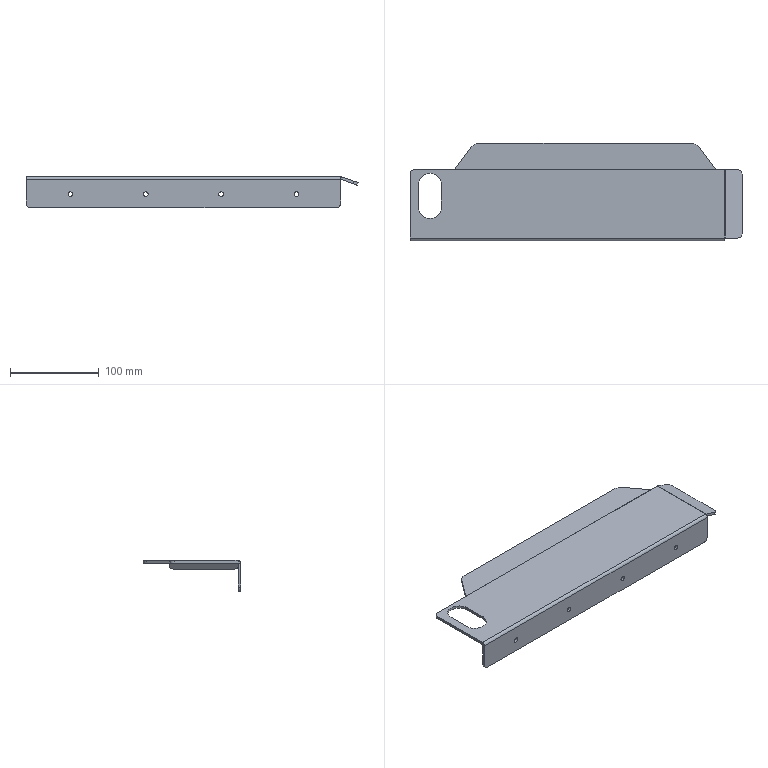Part | SolidWorks | features Fillet 3, ICE 3, EdgeFlange 1, ExtruThin 1, FlatPattern 1, FlattenBends 1, HoleWzd 1, ProcessBends 1, SheetMetal 1 | 2 solids | 48 faces | box 374.323 x 110 x 35 mm | volume 143786 mm3 | plane 27 | cylinder 21 | commonest cylinder face diameters 5.2 x8 10 x5 0.2 x2 6.2 x2 20 x2 26 x2
STEP:
#1=CARTESIAN_POINT('',(50.,0.,12.4));
#2=VERTEX_POINT('',#1);
#3=CARTESIAN_POINT('',(50.,0.,17.6));
#4=VERTEX_POINT('',#3);
#5=CARTESIAN_POINT('',(50.,0.,15.));
#6=DIRECTION('',(0.,1.,0.));
#7=DIRECTION('',(0.,0.,1.));
#8=AXIS2_PLACEMENT_3D('',#5,#6,#7);
#9=CIRCLE('',#8,2.6);
#10=EDGE_CURVE('',#2,#4,#9,.T.);
#11=ORIENTED_EDGE('',*,*,#10,.F.);
#12=CARTESIAN_POINT('',(50.,3.,12.4));
#13=VERTEX_POINT('',#12);
#14=CARTESIAN_POINT('',(50.,3.,12.4));
#15=DIRECTION('',(0.,1.,0.));
#16=VECTOR('',#15,1000.);
#17=LINE('',#14,#16);
#18=EDGE_CURVE('',#2,#13,#17,.T.);
#19=ORIENTED_EDGE('',*,*,#18,.T.);
#20=CARTESIAN_POINT('',(50.,3.,17.6));
#21=VERTEX_POINT('',#20);
#22=CARTESIAN_POINT('',(50.,3.,15.));
#23=DIRECTION('',(0.,1.,0.));
#24=DIRECTION('',(0.,0.,1.));
#25=AXIS2_PLACEMENT_3D('',#22,#23,#24);
#26=CIRCLE('',#25,2.6);
#27=EDGE_CURVE('',#13,#21,#26,.T.);
#28=ORIENTED_EDGE('',*,*,#27,.T.);
#29=CARTESIAN_POINT('',(50.,3.,17.6));
#30=DIRECTION('',(0.,1.,0.));
#31=VECTOR('',#30,1000.);
#32=LINE('',#29,#31);
#33=EDGE_CURVE('',#4,#21,#32,.T.);
#34=ORIENTED_EDGE('',*,*,#33,.F.);
#35=EDGE_LOOP('',(#11,#19,#28,#34));
#36=FACE_OUTER_BOUND('',#35,.T.);
#37=CARTESIAN_POINT('',(50.,3.,15.));
#38=DIRECTION('',(0.,1.,0.));
#39=DIRECTION('',(0.,0.,1.));
#40=AXIS2_PLACEMENT_3D('',#37,#38,#39);
#41=CYLINDRICAL_SURFACE('',#40,2.6);
#42=ADVANCED_FACE('',(#36),#41,.F.);
#43=CARTESIAN_POINT('',(135.,0.,12.4));
#44=VERTEX_POINT('',#43);
#45=CARTESIAN_POINT('',(135.,0.,17.6));
#46=VERTEX_POINT('',#45);
#47=CARTESIAN_POINT('',(135.,0.,15.));
#48=DIRECTION('',(0.,1.,0.));
#49=DIRECTION('',(0.,0.,1.));
#50=AXIS2_PLACEMENT_3D('',#47,#48,#49);
#51=CIRCLE('',#50,2.6);
#52=EDGE_CURVE('',#44,#46,#51,.T.);
#53=ORIENTED_EDGE('',*,*,#52,.F.);
#54=CARTESIAN_POINT('',(135.,3.,12.4));
#55=VERTEX_POINT('',#54);
#56=CARTESIAN_POINT('',(135.,3.,12.4));
#57=DIRECTION('',(0.,1.,0.));
#58=VECTOR('',#57,1000.);
#59=LINE('',#56,#58);
#60=EDGE_CURVE('',#44,#55,#59,.T.);
#61=ORIENTED_EDGE('',*,*,#60,.T.);
#62=CARTESIAN_POINT('',(135.,3.,17.6));
#63=VERTEX_POINT('',#62);
#64=CARTESIAN_POINT('',(135.,3.,15.));
#65=DIRECTION('',(0.,1.,0.));
#66=DIRECTION('',(0.,0.,1.));
#67=AXIS2_PLACEMENT_3D('',#64,#65,#66);
#68=CIRCLE('',#67,2.6);
#69=EDGE_CURVE('',#55,#63,#68,.T.);
#70=ORIENTED_EDGE('',*,*,#69,.T.);
#71=CARTESIAN_POINT('',(135.,3.,17.6));
#72=DIRECTION('',(0.,1.,0.));
#73=VECTOR('',#72,1000.);
#74=LINE('',#71,#73);
#75=EDGE_CURVE('',#46,#63,#74,.T.);
#76=ORIENTED_EDGE('',*,*,#75,.F.);
#77=EDGE_LOOP('',(#53,#61,#70,#76));
#78=FACE_OUTER_BOUND('',#77,.T.);
#79=CARTESIAN_POINT('',(135.,3.,15.));
#80=DIRECTION('',(0.,1.,0.));
#81=DIRECTION('',(0.,0.,1.));
#82=AXIS2_PLACEMENT_3D('',#79,#80,#81);
#83=CYLINDRICAL_SURFACE('',#82,2.6);
#84=ADVANCED_FACE('',(#78),#83,.F.);
#85=CARTESIAN_POINT('',(220.,0.,12.4));
#86=VERTEX_POINT('',#85);
#87=CARTESIAN_POINT('',(220.,0.,17.6));
#88=VERTEX_POINT('',#87);
#89=CARTESIAN_POINT('',(220.,0.,15.));
#90=DIRECTION('',(0.,1.,0.));
#91=DIRECTION('',(0.,0.,1.));
#92=AXIS2_PLACEMENT_3D('',#89,#90,#91);
#93=CIRCLE('',#92,2.6);
#94=EDGE_CURVE('',#86,#88,#93,.T.);
#95=ORIENTED_EDGE('',*,*,#94,.F.);
#96=CARTESIAN_POINT('',(220.,3.,12.4));
#97=VERTEX_POINT('',#96);
#98=CARTESIAN_POINT('',(220.,3.,12.4));
#99=DIRECTION('',(0.,1.,0.));
#100=VECTOR('',#99,1000.);
#101=LINE('',#98,#100);
#102=EDGE_CURVE('',#86,#97,#101,.T.);
#103=ORIENTED_EDGE('',*,*,#102,.T.);
#104=CARTESIAN_POINT('',(220.,3.,17.6));
#105=VERTEX_POINT('',#104);
#106=CARTESIAN_POINT('',(220.,3.,15.));
#107=DIRECTION('',(0.,1.,0.));
#108=DIRECTION('',(0.,0.,1.));
#109=AXIS2_PLACEMENT_3D('',#106,#107,#108);
#110=CIRCLE('',#109,2.6);
#111=EDGE_CURVE('',#97,#105,#110,.T.);
#112=ORIENTED_EDGE('',*,*,#111,.T.);
#113=CARTESIAN_POINT('',(220.,3.,17.6));
#114=DIRECTION('',(0.,1.,0.));
#115=VECTOR('',#114,1000.);
#116=LINE('',#113,#115);
#117=EDGE_CURVE('',#88,#105,#116,.T.);
#118=ORIENTED_EDGE('',*,*,#117,.F.);
#119=EDGE_LOOP('',(#95,#103,#112,#118));
#120=FACE_OUTER_BOUND('',#119,.T.);
#121=CARTESIAN_POINT('',(220.,3.,15.));
#122=DIRECTION('',(0.,1.,0.));
#123=DIRECTION('',(0.,0.,1.));
#124=AXIS2_PLACEMENT_3D('',#121,#122,#123);
#125=CYLINDRICAL_SURFACE('',#124,2.6);
#126=ADVANCED_FACE('',(#120),#125,.F.);
#127=CARTESIAN_POINT('',(305.,0.,12.4));
#128=VERTEX_POINT('',#127);
#129=CARTESIAN_POINT('',(305.,0.,17.6));
#130=VERTEX_POINT('',#129);
#131=CARTESIAN_POINT('',(305.,0.,15.));
#132=DIRECTION('',(0.,1.,0.));
#133=DIRECTION('',(0.,0.,1.));
#134=AXIS2_PLACEMENT_3D('',#131,#132,#133);
#135=CIRCLE('',#134,2.6);
#136=EDGE_CURVE('',#128,#130,#135,.T.);
#137=ORIENTED_EDGE('',*,*,#136,.F.);
#138=CARTESIAN_POINT('',(305.,3.,12.4));
#139=VERTEX_POINT('',#138);
#140=CARTESIAN_POINT('',(305.,3.,12.4));
#141=DIRECTION('',(0.,1.,0.));
#142=VECTOR('',#141,1000.);
#143=LINE('',#140,#142);
#144=EDGE_CURVE('',#128,#139,#143,.T.);
#145=ORIENTED_EDGE('',*,*,#144,.T.);
#146=CARTESIAN_POINT('',(305.,3.,17.6));
#147=VERTEX_POINT('',#146);
#148=CARTESIAN_POINT('',(305.,3.,15.));
#149=DIRECTION('',(0.,1.,0.));
#150=DIRECTION('',(0.,0.,1.));
#151=AXIS2_PLACEMENT_3D('',#148,#149,#150);
#152=CIRCLE('',#151,2.6);
#153=EDGE_CURVE('',#139,#147,#152,.T.);
#154=ORIENTED_EDGE('',*,*,#153,.T.);
#155=CARTESIAN_POINT('',(305.,3.,17.6));
#156=DIRECTION('',(0.,1.,0.));
#157=VECTOR('',#156,1000.);
#158=LINE('',#155,#157);
#159=EDGE_CURVE('',#130,#147,#158,.T.);
#160=ORIENTED_EDGE('',*,*,#159,.F.);
#161=EDGE_LOOP('',(#137,#145,#154,#160));
#162=FACE_OUTER_BOUND('',#161,.T.);
#163=CARTESIAN_POINT('',(305.,3.,15.));
#164=DIRECTION('',(0.,1.,0.));
#165=DIRECTION('',(0.,0.,1.));
#166=AXIS2_PLACEMENT_3D('',#163,#164,#165);
#167=CYLINDRICAL_SURFACE('',#166,2.6);
#168=ADVANCED_FACE('',(#162),#167,.F.);
#169=CARTESIAN_POINT('',(354.982,0.,31.9));
#170=VERTEX_POINT('',#169);
#171=CARTESIAN_POINT('',(354.982,3.,31.9));
#172=VERTEX_POINT('',#171);
#173=CARTESIAN_POINT('',(354.982,0.,31.9));
#174=DIRECTION('',(0.,1.,0.));
#175=VECTOR('',#174,1000.);
#176=LINE('',#173,#175);
#177=EDGE_CURVE('',#170,#172,#176,.T.);
#178=ORIENTED_EDGE('',*,*,#177,.F.);
#179=CARTESIAN_POINT('',(355.,0.,31.9));
#180=VERTEX_POINT('',#179);
#181=CARTESIAN_POINT('',(355.,0.,31.9));
#182=DIRECTION('',(1.,0.,0.));
#183=VECTOR('',#182,1000.);
#184=LINE('',#181,#183);
#185=EDGE_CURVE('',#170,#180,#184,.T.);
#186=ORIENTED_EDGE('',*,*,#185,.T.);
#187=CARTESIAN_POINT('',(355.,3.,31.9));
#188=VERTEX_POINT('',#187);
#189=CARTESIAN_POINT('',(355.,712.861,31.9));
#190=DIRECTION('',(0.,-1.,0.));
#191=VECTOR('',#190,1000.);
#192=LINE('',#189,#191);
#193=EDGE_CURVE('',#188,#180,#192,.T.);
#194=ORIENTED_EDGE('',*,*,#193,.F.);
#195=CARTESIAN_POINT('',(355.,3.,31.9));
#196=DIRECTION('',(1.,0.,0.));
#197=VECTOR('',#196,1000.);
#198=LINE('',#195,#197);
#199=EDGE_CURVE('',#172,#188,#198,.T.);
#200=ORIENTED_EDGE('',*,*,#199,.F.);
#201=EDGE_LOOP('',(#178,#186,#194,#200));
#202=FACE_OUTER_BOUND('',#201,.T.);
#203=CARTESIAN_POINT('',(0.,0.,31.9));
#204=DIRECTION('',(0.,0.,-1.));
#205=DIRECTION('',(-1.,0.,0.));
#206=AXIS2_PLACEMENT_3D('',#203,#204,#205);
#207=PLANE('',#206);
#208=ADVANCED_FACE('',(#202),#207,.F.);
#209=CARTESIAN_POINT('',(0.,0.,31.9));
#210=VERTEX_POINT('',#209);
#211=CARTESIAN_POINT('',(355.,0.,31.9));
#212=DIRECTION('',(1.,0.,0.));
#213=VECTOR('',#212,1000.);
#214=LINE('',#211,#213);
#215=EDGE_CURVE('',#210,#170,#214,.T.);
#216=ORIENTED_EDGE('',*,*,#215,.T.);
#217=CARTESIAN_POINT('',(354.982,3.1,35.));
#218=VERTEX_POINT('',#217);
#219=CARTESIAN_POINT('',(354.982,3.1,31.9));
#220=DIRECTION('',(-1.,0.,0.));
#221=DIRECTION('',(0.,0.,-1.));
#222=AXIS2_PLACEMENT_3D('',#219,#220,#221);
#223=CIRCLE('',#222,3.1);
#224=EDGE_CURVE('',#170,#218,#223,.T.);
#225=ORIENTED_EDGE('',*,*,#224,.T.);
#226=CARTESIAN_POINT('',(0.,3.1,35.));
#227=VERTEX_POINT('',#226);
#228=CARTESIAN_POINT('',(355.,3.1,35.));
#229=DIRECTION('',(1.,0.,0.));
#230=VECTOR('',#229,1000.);
#231=LINE('',#228,#230);
#232=EDGE_CURVE('',#227,#218,#231,.T.);
#233=ORIENTED_EDGE('',*,*,#232,.F.);
#234=CARTESIAN_POINT('',(0.,3.1,31.9));
#235=DIRECTION('',(1.,0.,0.));
#236=DIRECTION('',(0.,0.,1.));
#237=AXIS2_PLACEMENT_3D('',#234,#235,#236);
#238=CIRCLE('',#237,3.1);
#239=EDGE_CURVE('',#227,#210,#238,.T.);
#240=ORIENTED_EDGE('',*,*,#239,.T.);
#241=EDGE_LOOP('',(#216,#225,#233,#240));
#242=FACE_OUTER_BOUND('',#241,.T.);
#243=CARTESIAN_POINT('',(726.664,3.1,31.9));
#244=DIRECTION('',(-1.,0.,0.));
#245=DIRECTION('',(0.,0.,1.));
#246=AXIS2_PLACEMENT_3D('',#243,#244,#245);
#247=CYLINDRICAL_SURFACE('',#246,3.1);
#248=ADVANCED_FACE('',(#242),#247,.T.);
#249=CARTESIAN_POINT('',(9.5,38.,32.));
#250=VERTEX_POINT('',#249);
#251=CARTESIAN_POINT('',(9.5,63.,32.));
#252=VERTEX_POINT('',#251);
#253=CARTESIAN_POINT('',(9.5,38.,32.));
#254=DIRECTION('',(0.,1.,0.));
#255=VECTOR('',#254,1000.);
#256=LINE('',#253,#255);
#257=EDGE_CURVE('',#250,#252,#256,.T.);
#258=ORIENTED_EDGE('',*,*,#257,.F.);
#259=CARTESIAN_POINT('',(35.5,38.,32.));
#260=VERTEX_POINT('',#259);
#261=CARTESIAN_POINT('',(22.5,38.,32.));
#262=DIRECTION('',(0.,0.,-1.));
#263=DIRECTION('',(-1.,0.,0.));
#264=AXIS2_PLACEMENT_3D('',#261,#262,#263);
#265=CIRCLE('',#264,13.);
#266=EDGE_CURVE('',#260,#250,#265,.T.);
#267=ORIENTED_EDGE('',*,*,#266,.F.);
#268=CARTESIAN_POINT('',(35.5,63.,32.));
#269=VERTEX_POINT('',#268);
#270=CARTESIAN_POINT('',(35.5,38.,32.));
#271=DIRECTION('',(0.,-1.,0.));
#272=VECTOR('',#271,1000.);
#273=LINE('',#270,#272);
#274=EDGE_CURVE('',#269,#260,#273,.T.);
#275=ORIENTED_EDGE('',*,*,#274,.F.);
#276=CARTESIAN_POINT('',(22.5,63.,32.));
#277=DIRECTION('',(0.,0.,-1.));
#278=DIRECTION('',(-1.,0.,0.));
#279=AXIS2_PLACEMENT_3D('',#276,#277,#278);
#280=CIRCLE('',#279,13.);
#281=EDGE_CURVE('',#252,#269,#280,.T.);
#282=ORIENTED_EDGE('',*,*,#281,.F.);
#283=EDGE_LOOP('',(#258,#267,#275,#282));
#284=FACE_BOUND('',#283,.T.);
#285=CARTESIAN_POINT('',(354.982,3.1,32.));
#286=VERTEX_POINT('',#285);
#287=CARTESIAN_POINT('',(354.982,80.,32.));
#288=VERTEX_POINT('',#287);
#289=CARTESIAN_POINT('',(354.982,3.1,32.));
#290=DIRECTION('',(0.,1.,0.));
#291=VECTOR('',#290,1000.);
#292=LINE('',#289,#291);
#293=EDGE_CURVE('',#286,#288,#292,.T.);
#294=ORIENTED_EDGE('',*,*,#293,.F.);
#295=CARTESIAN_POINT('',(0.,3.1,32.));
#296=VERTEX_POINT('',#295);
#297=CARTESIAN_POINT('',(355.,3.1,32.));
#298=DIRECTION('',(1.,0.,0.));
#299=VECTOR('',#298,1000.);
#300=LINE('',#297,#299);
#301=EDGE_CURVE('',#296,#286,#300,.T.);
#302=ORIENTED_EDGE('',*,*,#301,.F.);
#303=CARTESIAN_POINT('',(0.,75.,32.));
#304=VERTEX_POINT('',#303);
#305=CARTESIAN_POINT('',(0.,0.,32.));
#306=DIRECTION('',(0.,1.,0.));
#307=VECTOR('',#306,1000.);
#308=LINE('',#305,#307);
#309=EDGE_CURVE('',#296,#304,#308,.T.);
#310=ORIENTED_EDGE('',*,*,#309,.T.);
#311=CARTESIAN_POINT('',(5.,80.,32.));
#312=VERTEX_POINT('',#311);
#313=CARTESIAN_POINT('',(5.,75.,32.));
#314=DIRECTION('',(0.,0.,-1.));
#315=DIRECTION('',(1.,0.,0.));
#316=AXIS2_PLACEMENT_3D('',#313,#314,#315);
#317=CIRCLE('',#316,5.);
#318=EDGE_CURVE('',#304,#312,#317,.T.);
#319=ORIENTED_EDGE('',*,*,#318,.T.);
#320=CARTESIAN_POINT('',(355.,80.,32.));
#321=DIRECTION('',(-1.,0.,0.));
#322=VECTOR('',#321,1000.);
#323=LINE('',#320,#322);
#324=EDGE_CURVE('',#288,#312,#323,.T.);
#325=ORIENTED_EDGE('',*,*,#324,.F.);
#326=EDGE_LOOP('',(#294,#302,#310,#319,#325));
#327=FACE_OUTER_BOUND('',#326,.T.);
#328=CARTESIAN_POINT('',(355.,0.,32.));
#329=DIRECTION('',(0.,0.,1.));
#330=DIRECTION('',(1.,0.,0.));
#331=AXIS2_PLACEMENT_3D('',#328,#329,#330);
#332=PLANE('',#331);
#333=ADVANCED_FACE('',(#284,#327),#332,.F.);
#334=CARTESIAN_POINT('',(35.5,38.,35.));
#335=VERTEX_POINT('',#334);
#336=CARTESIAN_POINT('',(9.5,38.,35.));
#337=VERTEX_POINT('',#336);
#338=CARTESIAN_POINT('',(22.5,38.,35.));
#339=DIRECTION('',(0.,0.,-1.));
#340=DIRECTION('',(-1.,0.,0.));
#341=AXIS2_PLACEMENT_3D('',#338,#339,#340);
#342=CIRCLE('',#341,13.);
#343=EDGE_CURVE('',#335,#337,#342,.T.);
#344=ORIENTED_EDGE('',*,*,#343,.T.);
#345=CARTESIAN_POINT('',(9.5,63.,35.));
#346=VERTEX_POINT('',#345);
#347=CARTESIAN_POINT('',(9.5,38.,35.));
#348=DIRECTION('',(0.,1.,0.));
#349=VECTOR('',#348,1000.);
#350=LINE('',#347,#349);
#351=EDGE_CURVE('',#337,#346,#350,.T.);
#352=ORIENTED_EDGE('',*,*,#351,.T.);
#353=CARTESIAN_POINT('',(35.5,63.,35.));
#354=VERTEX_POINT('',#353);
#355=CARTESIAN_POINT('',(22.5,63.,35.));
#356=DIRECTION('',(0.,0.,-1.));
#357=DIRECTION('',(-1.,0.,0.));
#358=AXIS2_PLACEMENT_3D('',#355,#356,#357);
#359=CIRCLE('',#358,13.);
#360=EDGE_CURVE('',#346,#354,#359,.T.);
#361=ORIENTED_EDGE('',*,*,#360,.T.);
#362=CARTESIAN_POINT('',(35.5,38.,35.));
#363=DIRECTION('',(0.,-1.,0.));
#364=VECTOR('',#363,1000.);
#365=LINE('',#362,#364);
#366=EDGE_CURVE('',#354,#335,#365,.T.);
#367=ORIENTED_EDGE('',*,*,#366,.T.);
#368=EDGE_LOOP('',(#344,#352,#361,#367));
#369=FACE_BOUND('',#368,.T.);
#370=ORIENTED_EDGE('',*,*,#232,.T.);
#371=CARTESIAN_POINT('',(354.982,80.,35.));
#372=VERTEX_POINT('',#371);
#373=CARTESIAN_POINT('',(354.982,3.1,35.));
#374=DIRECTION('',(0.,1.,0.));
#375=VECTOR('',#374,1000.);
#376=LINE('',#373,#375);
#377=EDGE_CURVE('',#218,#372,#376,.T.);
#378=ORIENTED_EDGE('',*,*,#377,.T.);
#379=CARTESIAN_POINT('',(5.,80.,35.));
#380=VERTEX_POINT('',#379);
#381=CARTESIAN_POINT('',(355.,80.,35.));
#382=DIRECTION('',(-1.,0.,0.));
#383=VECTOR('',#382,1000.);
#384=LINE('',#381,#383);
#385=EDGE_CURVE('',#372,#380,#384,.T.);
#386=ORIENTED_EDGE('',*,*,#385,.T.);
#387=CARTESIAN_POINT('',(0.,75.,35.));
#388=VERTEX_POINT('',#387);
#389=CARTESIAN_POINT('',(5.,75.,35.));
#390=DIRECTION('',(0.,0.,1.));
#391=DIRECTION('',(1.,0.,0.));
#392=AXIS2_PLACEMENT_3D('',#389,#390,#391);
#393=CIRCLE('',#392,5.);
#394=EDGE_CURVE('',#380,#388,#393,.T.);
#395=ORIENTED_EDGE('',*,*,#394,.T.);
#396=CARTESIAN_POINT('',(0.,0.,35.));
#397=DIRECTION('',(0.,1.,0.));
#398=VECTOR('',#397,1000.);
#399=LINE('',#396,#398);
#400=EDGE_CURVE('',#227,#388,#399,.T.);
#401=ORIENTED_EDGE('',*,*,#400,.F.);
#402=EDGE_LOOP('',(#370,#378,#386,#395,#401));
#403=FACE_OUTER_BOUND('',#402,.T.);
#404=CARTESIAN_POINT('',(355.,0.,35.));
#405=DIRECTION('',(0.,0.,1.));
#406=DIRECTION('',(1.,0.,0.));
#407=AXIS2_PLACEMENT_3D('',#404,#405,#406);
#408=PLANE('',#407);
#409=ADVANCED_FACE('',(#369,#403),#408,.T.);
#410=ORIENTED_EDGE('',*,*,#144,.F.);
#411=CARTESIAN_POINT('',(305.,0.,15.));
#412=DIRECTION('',(0.,1.,0.));
#413=DIRECTION('',(0.,0.,1.));
#414=AXIS2_PLACEMENT_3D('',#411,#412,#413);
#415=CIRCLE('',#414,2.6);
#416=EDGE_CURVE('',#130,#128,#415,.T.);
#417=ORIENTED_EDGE('',*,*,#416,.F.);
#418=ORIENTED_EDGE('',*,*,#159,.T.);
#419=CARTESIAN_POINT('',(305.,3.,15.));
#420=DIRECTION('',(0.,1.,0.));
#421=DIRECTION('',(0.,0.,1.));
#422=AXIS2_PLACEMENT_3D('',#419,#420,#421);
#423=CIRCLE('',#422,2.6);
#424=EDGE_CURVE('',#147,#139,#423,.T.);
#425=ORIENTED_EDGE('',*,*,#424,.T.);
#426=EDGE_LOOP('',(#410,#417,#418,#425));
#427=FACE_OUTER_BOUND('',#426,.T.);
#428=CARTESIAN_POINT('',(305.,3.,15.));
#429=DIRECTION('',(0.,1.,0.));
#430=DIRECTION('',(0.,0.,1.));
#431=AXIS2_PLACEMENT_3D('',#428,#429,#430);
#432=CYLINDRICAL_SURFACE('',#431,2.6);
#433=ADVANCED_FACE('',(#427),#432,.F.);
#434=ORIENTED_EDGE('',*,*,#102,.F.);
#435=CARTESIAN_POINT('',(220.,0.,15.));
#436=DIRECTION('',(0.,1.,0.));
#437=DIRECTION('',(0.,0.,1.));
#438=AXIS2_PLACEMENT_3D('',#435,#436,#437);
#439=CIRCLE('',#438,2.6);
#440=EDGE_CURVE('',#88,#86,#439,.T.);
#441=ORIENTED_EDGE('',*,*,#440,.F.);
#442=ORIENTED_EDGE('',*,*,#117,.T.);
#443=CARTESIAN_POINT('',(220.,3.,15.));
#444=DIRECTION('',(0.,1.,0.));
#445=DIRECTION('',(0.,0.,1.));
#446=AXIS2_PLACEMENT_3D('',#443,#444,#445);
#447=CIRCLE('',#446,2.6);
#448=EDGE_CURVE('',#105,#97,#447,.T.);
#449=ORIENTED_EDGE('',*,*,#448,.T.);
#450=EDGE_LOOP('',(#434,#441,#442,#449));
#451=FACE_OUTER_BOUND('',#450,.T.);
#452=CARTESIAN_POINT('',(220.,3.,15.));
#453=DIRECTION('',(0.,1.,0.));
#454=DIRECTION('',(0.,0.,1.));
#455=AXIS2_PLACEMENT_3D('',#452,#453,#454);
#456=CYLINDRICAL_SURFACE('',#455,2.6);
#457=ADVANCED_FACE('',(#451),#456,.F.);
#458=ORIENTED_EDGE('',*,*,#60,.F.);
#459=CARTESIAN_POINT('',(135.,0.,15.));
#460=DIRECTION('',(0.,1.,0.));
#461=DIRECTION('',(0.,0.,1.));
#462=AXIS2_PLACEMENT_3D('',#459,#460,#461);
#463=CIRCLE('',#462,2.6);
#464=EDGE_CURVE('',#46,#44,#463,.T.);
#465=ORIENTED_EDGE('',*,*,#464,.F.);
#466=ORIENTED_EDGE('',*,*,#75,.T.);
#467=CARTESIAN_POINT('',(135.,3.,15.));
#468=DIRECTION('',(0.,1.,0.));
#469=DIRECTION('',(0.,0.,1.));
#470=AXIS2_PLACEMENT_3D('',#467,#468,#469);
#471=CIRCLE('',#470,2.6);
#472=EDGE_CURVE('',#63,#55,#471,.T.);
#473=ORIENTED_EDGE('',*,*,#472,.T.);
#474=EDGE_LOOP('',(#458,#465,#466,#473));
#475=FACE_OUTER_BOUND('',#474,.T.);
#476=CARTESIAN_POINT('',(135.,3.,15.));
#477=DIRECTION('',(0.,1.,0.));
#478=DIRECTION('',(0.,0.,1.));
#479=AXIS2_PLACEMENT_3D('',#476,#477,#478);
#480=CYLINDRICAL_SURFACE('',#479,2.6);
#481=ADVANCED_FACE('',(#475),#480,.F.);
#482=ORIENTED_EDGE('',*,*,#18,.F.);
#483=CARTESIAN_POINT('',(50.,0.,15.));
#484=DIRECTION('',(0.,1.,0.));
#485=DIRECTION('',(0.,0.,1.));
#486=AXIS2_PLACEMENT_3D('',#483,#484,#485);
#487=CIRCLE('',#486,2.6);
#488=EDGE_CURVE('',#4,#2,#487,.T.);
#489=ORIENTED_EDGE('',*,*,#488,.F.);
#490=ORIENTED_EDGE('',*,*,#33,.T.);
#491=CARTESIAN_POINT('',(50.,3.,15.));
#492=DIRECTION('',(0.,1.,0.));
#493=DIRECTION('',(0.,0.,1.));
#494=AXIS2_PLACEMENT_3D('',#491,#492,#493);
#495=CIRCLE('',#494,2.6);
#496=EDGE_CURVE('',#21,#13,#495,.T.);
#497=ORIENTED_EDGE('',*,*,#496,.T.);
#498=EDGE_LOOP('',(#482,#489,#490,#497));
#499=FACE_OUTER_BOUND('',#498,.T.);
#500=CARTESIAN_POINT('',(50.,3.,15.));
#501=DIRECTION('',(0.,1.,0.));
#502=DIRECTION('',(0.,0.,1.));
#503=AXIS2_PLACEMENT_3D('',#500,#501,#502);
#504=CYLINDRICAL_SURFACE('',#503,2.6);
#505=ADVANCED_FACE('',(#499),#504,.F.);
#506=CARTESIAN_POINT('',(350.,0.,0.));
#507=VERTEX_POINT('',#506);
#508=CARTESIAN_POINT('',(5.,0.,0.));
#509=VERTEX_POINT('',#508);
#510=CARTESIAN_POINT('',(355.,0.,0.));
#511=DIRECTION('',(-1.,0.,0.));
#512=VECTOR('',#511,1000.);
#513=LINE('',#510,#512);
#514=EDGE_CURVE('',#507,#509,#513,.T.);
#515=ORIENTED_EDGE('',*,*,#514,.T.);
#516=CARTESIAN_POINT('',(5.,3.,0.));
#517=VERTEX_POINT('',#516);
#518=CARTESIAN_POINT('',(5.,712.861,0.));
#519=DIRECTION('',(0.,-1.,0.));
#520=VECTOR('',#519,1000.);
#521=LINE('',#518,#520);
#522=EDGE_CURVE('',#517,#509,#521,.T.);
#523=ORIENTED_EDGE('',*,*,#522,.F.);
#524=CARTESIAN_POINT('',(350.,3.,0.));
#525=VERTEX_POINT('',#524);
#526=CARTESIAN_POINT('',(355.,3.,0.));
#527=DIRECTION('',(-1.,0.,0.));
#528=VECTOR('',#527,1000.);
#529=LINE('',#526,#528);
#530=EDGE_CURVE('',#525,#517,#529,.T.);
#531=ORIENTED_EDGE('',*,*,#530,.F.);
#532=CARTESIAN_POINT('',(350.,712.861,0.));
#533=DIRECTION('',(0.,-1.,0.));
#534=VECTOR('',#533,1000.);
#535=LINE('',#532,#534);
#536=EDGE_CURVE('',#525,#507,#535,.T.);
#537=ORIENTED_EDGE('',*,*,#536,.T.);
#538=EDGE_LOOP('',(#515,#523,#531,#537));
#539=FACE_OUTER_BOUND('',#538,.T.);
#540=CARTESIAN_POINT('',(355.,712.861,0.));
#541=DIRECTION('',(0.,0.,1.));
#542=DIRECTION('',(0.,-1.,0.));
#543=AXIS2_PLACEMENT_3D('',#540,#541,#542);
#544=PLANE('',#543);
#545=ADVANCED_FACE('',(#539),#544,.F.);
#546=CARTESIAN_POINT('',(0.,0.,5.));
#547=VERTEX_POINT('',#546);
#548=CARTESIAN_POINT('',(5.,0.,5.));
#549=DIRECTION('',(0.,-1.,0.));
#550=DIRECTION('',(0.,0.,-1.));
#551=AXIS2_PLACEMENT_3D('',#548,#549,#550);
#552=CIRCLE('',#551,5.);
#553=EDGE_CURVE('',#547,#509,#552,.T.);
#554=ORIENTED_EDGE('',*,*,#553,.F.);
#555=CARTESIAN_POINT('',(0.,3.,5.));
#556=VERTEX_POINT('',#555);
#557=CARTESIAN_POINT('',(0.,712.861,5.));
#558=DIRECTION('',(0.,-1.,0.));
#559=VECTOR('',#558,1000.);
#560=LINE('',#557,#559);
#561=EDGE_CURVE('',#556,#547,#560,.T.);
#562=ORIENTED_EDGE('',*,*,#561,.F.);
#563=CARTESIAN_POINT('',(5.,3.,5.));
#564=DIRECTION('',(0.,1.,0.));
#565=DIRECTION('',(0.,0.,-1.));
#566=AXIS2_PLACEMENT_3D('',#563,#564,#565);
#567=CIRCLE('',#566,5.);
#568=EDGE_CURVE('',#517,#556,#567,.T.);
#569=ORIENTED_EDGE('',*,*,#568,.F.);
#570=ORIENTED_EDGE('',*,*,#522,.T.);
#571=EDGE_LOOP('',(#554,#562,#569,#570));
#572=FACE_OUTER_BOUND('',#571,.T.);
#573=CARTESIAN_POINT('',(5.,712.861,5.));
#574=DIRECTION('',(0.,-1.,0.));
#575=DIRECTION('',(0.,0.,-1.));
#576=AXIS2_PLACEMENT_3D('',#573,#574,#575);
#577=CYLINDRICAL_SURFACE('',#576,5.);
#578=ADVANCED_FACE('',(#572),#577,.T.);
#579=CARTESIAN_POINT('',(355.,0.,5.));
#580=VERTEX_POINT('',#579);
#581=CARTESIAN_POINT('',(350.,0.,5.));
#582=DIRECTION('',(0.,-1.,0.));
#583=DIRECTION('',(0.,0.,-1.));
#584=AXIS2_PLACEMENT_3D('',#581,#582,#583);
#585=CIRCLE('',#584,5.);
#586=EDGE_CURVE('',#507,#580,#585,.T.);
#587=ORIENTED_EDGE('',*,*,#586,.F.);
#588=ORIENTED_EDGE('',*,*,#536,.F.);
#589=CARTESIAN_POINT('',(355.,3.,5.));
#590=VERTEX_POINT('',#589);
#591=CARTESIAN_POINT('',(350.,3.,5.));
#592=DIRECTION('',(0.,1.,0.));
#593=DIRECTION('',(0.,0.,-1.));
#594=AXIS2_PLACEMENT_3D('',#591,#592,#593);
#595=CIRCLE('',#594,5.);
#596=EDGE_CURVE('',#590,#525,#595,.T.);
#597=ORIENTED_EDGE('',*,*,#596,.F.);
#598=CARTESIAN_POINT('',(355.,712.861,5.));
#599=DIRECTION('',(0.,-1.,0.));
#600=VECTOR('',#599,1000.);
#601=LINE('',#598,#600);
#602=EDGE_CURVE('',#590,#580,#601,.T.);
#603=ORIENTED_EDGE('',*,*,#602,.T.);
#604=EDGE_LOOP('',(#587,#588,#597,#603));
#605=FACE_OUTER_BOUND('',#604,.T.);
#606=CARTESIAN_POINT('',(350.,712.861,5.));
#607=DIRECTION('',(0.,-1.,0.));
#608=DIRECTION('',(0.,0.,-1.));
#609=AXIS2_PLACEMENT_3D('',#606,#607,#608);
#610=CYLINDRICAL_SURFACE('',#609,5.);
#611=ADVANCED_FACE('',(#605),#610,.T.);
#612=ORIENTED_EDGE('',*,*,#193,.T.);
#613=CARTESIAN_POINT('',(355.,0.,0.));
#614=DIRECTION('',(0.,0.,1.));
#615=VECTOR('',#614,1000.);
#616=LINE('',#613,#615);
#617=EDGE_CURVE('',#580,#180,#616,.T.);
#618=ORIENTED_EDGE('',*,*,#617,.F.);
#619=ORIENTED_EDGE('',*,*,#602,.F.);
#620=CARTESIAN_POINT('',(355.,3.,0.));
#621=DIRECTION('',(0.,0.,1.));
#622=VECTOR('',#621,1000.);
#623=LINE('',#620,#622);
#624=EDGE_CURVE('',#590,#188,#623,.T.);
#625=ORIENTED_EDGE('',*,*,#624,.T.);
#626=EDGE_LOOP('',(#612,#618,#619,#625));
#627=FACE_OUTER_BOUND('',#626,.T.);
#628=CARTESIAN_POINT('',(355.,712.861,0.));
#629=DIRECTION('',(1.,0.,0.));
#630=DIRECTION('',(0.,1.,0.));
#631=AXIS2_PLACEMENT_3D('',#628,#629,#630);
#632=PLANE('',#631);
#633=ADVANCED_FACE('',(#627),#632,.T.);
#634=ORIENTED_EDGE('',*,*,#215,.F.);
#635=CARTESIAN_POINT('',(0.,0.,0.));
#636=DIRECTION('',(0.,0.,1.));
#637=VECTOR('',#636,1000.);
#638=LINE('',#635,#637);
#639=EDGE_CURVE('',#547,#210,#638,.T.);
#640=ORIENTED_EDGE('',*,*,#639,.F.);
#641=ORIENTED_EDGE('',*,*,#553,.T.);
#642=ORIENTED_EDGE('',*,*,#514,.F.);
#643=ORIENTED_EDGE('',*,*,#586,.T.);
#644=ORIENTED_EDGE('',*,*,#617,.T.);
#645=ORIENTED_EDGE('',*,*,#185,.F.);
#646=EDGE_LOOP('',(#634,#640,#641,#642,#643,#644,#645));
#647=FACE_OUTER_BOUND('',#646,.T.);
#648=ORIENTED_EDGE('',*,*,#488,.T.);
#649=ORIENTED_EDGE('',*,*,#10,.T.);
#650=EDGE_LOOP('',(#648,#649));
#651=FACE_BOUND('',#650,.T.);
#652=ORIENTED_EDGE('',*,*,#464,.T.);
#653=ORIENTED_EDGE('',*,*,#52,.T.);
#654=EDGE_LOOP('',(#652,#653));
#655=FACE_BOUND('',#654,.T.);
#656=ORIENTED_EDGE('',*,*,#440,.T.);
#657=ORIENTED_EDGE('',*,*,#94,.T.);
#658=EDGE_LOOP('',(#656,#657));
#659=FACE_BOUND('',#658,.T.);
#660=ORIENTED_EDGE('',*,*,#416,.T.);
#661=ORIENTED_EDGE('',*,*,#136,.T.);
#662=EDGE_LOOP('',(#660,#661));
#663=FACE_BOUND('',#662,.T.);
#664=CARTESIAN_POINT('',(355.,0.,0.));
#665=DIRECTION('',(0.,-1.,0.));
#666=DIRECTION('',(0.,0.,-1.));
#667=AXIS2_PLACEMENT_3D('',#664,#665,#666);
#668=PLANE('',#667);
#669=ADVANCED_FACE('',(#647,#651,#655,#659,#663),#668,.T.);
#670=ORIENTED_EDGE('',*,*,#639,.T.);
#671=CARTESIAN_POINT('',(0.,3.,31.9));
#672=VERTEX_POINT('',#671);
#673=CARTESIAN_POINT('',(0.,712.861,31.9));
#674=DIRECTION('',(0.,-1.,0.));
#675=VECTOR('',#674,1000.);
#676=LINE('',#673,#675);
#677=EDGE_CURVE('',#672,#210,#676,.T.);
#678=ORIENTED_EDGE('',*,*,#677,.F.);
#679=CARTESIAN_POINT('',(0.,3.,0.));
#680=DIRECTION('',(0.,0.,1.));
#681=VECTOR('',#680,1000.);
#682=LINE('',#679,#681);
#683=EDGE_CURVE('',#556,#672,#682,.T.);
#684=ORIENTED_EDGE('',*,*,#683,.F.);
#685=ORIENTED_EDGE('',*,*,#561,.T.);
#686=EDGE_LOOP('',(#670,#678,#684,#685));
#687=FACE_OUTER_BOUND('',#686,.T.);
#688=CARTESIAN_POINT('',(0.,712.861,0.));
#689=DIRECTION('',(1.,0.,0.));
#690=DIRECTION('',(0.,1.,0.));
#691=AXIS2_PLACEMENT_3D('',#688,#689,#690);
#692=PLANE('',#691);
#693=ADVANCED_FACE('',(#687),#692,.F.);
#694=ORIENTED_EDGE('',*,*,#496,.F.);
#695=ORIENTED_EDGE('',*,*,#27,.F.);
#696=EDGE_LOOP('',(#694,#695));
#697=FACE_BOUND('',#696,.T.);
#698=ORIENTED_EDGE('',*,*,#472,.F.);
#699=ORIENTED_EDGE('',*,*,#69,.F.);
#700=EDGE_LOOP('',(#698,#699));
#701=FACE_BOUND('',#700,.T.);
#702=ORIENTED_EDGE('',*,*,#448,.F.);
#703=ORIENTED_EDGE('',*,*,#111,.F.);
#704=EDGE_LOOP('',(#702,#703));
#705=FACE_BOUND('',#704,.T.);
#706=ORIENTED_EDGE('',*,*,#424,.F.);
#707=ORIENTED_EDGE('',*,*,#153,.F.);
#708=EDGE_LOOP('',(#706,#707));
#709=FACE_BOUND('',#708,.T.);
#710=ORIENTED_EDGE('',*,*,#683,.T.);
#711=CARTESIAN_POINT('',(355.,3.,31.9));
#712=DIRECTION('',(1.,0.,0.));
#713=VECTOR('',#712,1000.);
#714=LINE('',#711,#713);
#715=EDGE_CURVE('',#672,#172,#714,.T.);
#716=ORIENTED_EDGE('',*,*,#715,.T.);
#717=ORIENTED_EDGE('',*,*,#199,.T.);
#718=ORIENTED_EDGE('',*,*,#624,.F.);
#719=ORIENTED_EDGE('',*,*,#596,.T.);
#720=ORIENTED_EDGE('',*,*,#530,.T.);
#721=ORIENTED_EDGE('',*,*,#568,.T.);
#722=EDGE_LOOP('',(#710,#716,#717,#718,#719,#720,#721));
#723=FACE_OUTER_BOUND('',#722,.T.);
#724=CARTESIAN_POINT('',(355.,3.,0.));
#725=DIRECTION('',(0.,-1.,0.));
#726=DIRECTION('',(0.,0.,-1.));
#727=AXIS2_PLACEMENT_3D('',#724,#725,#726);
#728=PLANE('',#727);
#729=ADVANCED_FACE('',(#697,#701,#705,#709,#723),#728,.F.);
#730=ORIENTED_EDGE('',*,*,#400,.T.);
#731=CARTESIAN_POINT('',(0.,75.,-691.467));
#732=DIRECTION('',(0.,0.,1.));
#733=VECTOR('',#732,1000.);
#734=LINE('',#731,#733);
#735=EDGE_CURVE('',#304,#388,#734,.T.);
#736=ORIENTED_EDGE('',*,*,#735,.F.);
#737=ORIENTED_EDGE('',*,*,#309,.F.);
#738=CARTESIAN_POINT('',(0.,3.1,-691.467));
#739=DIRECTION('',(0.,0.,1.));
#740=VECTOR('',#739,1000.);
#741=LINE('',#738,#740);
#742=EDGE_CURVE('',#296,#227,#741,.T.);
#743=ORIENTED_EDGE('',*,*,#742,.T.);
#744=EDGE_LOOP('',(#730,#736,#737,#743));
#745=FACE_OUTER_BOUND('',#744,.T.);
#746=CARTESIAN_POINT('',(0.,0.,-691.467));
#747=DIRECTION('',(1.,0.,0.));
#748=DIRECTION('',(0.,0.,-1.));
#749=AXIS2_PLACEMENT_3D('',#746,#747,#748);
#750=PLANE('',#749);
#751=ADVANCED_FACE('',(#745),#750,.F.);
#752=ORIENTED_EDGE('',*,*,#394,.F.);
#753=CARTESIAN_POINT('',(5.,80.,-691.467));
#754=DIRECTION('',(0.,0.,1.));
#755=VECTOR('',#754,1000.);
#756=LINE('',#753,#755);
#757=EDGE_CURVE('',#312,#380,#756,.T.);
#758=ORIENTED_EDGE('',*,*,#757,.F.);
#759=ORIENTED_EDGE('',*,*,#318,.F.);
#760=ORIENTED_EDGE('',*,*,#735,.T.);
#761=EDGE_LOOP('',(#752,#758,#759,#760));
#762=FACE_OUTER_BOUND('',#761,.T.);
#763=CARTESIAN_POINT('',(5.,75.,-691.467));
#764=DIRECTION('',(0.,0.,1.));
#765=DIRECTION('',(1.,0.,0.));
#766=AXIS2_PLACEMENT_3D('',#763,#764,#765);
#767=CYLINDRICAL_SURFACE('',#766,5.);
#768=ADVANCED_FACE('',(#762),#767,.T.);
#769=CARTESIAN_POINT('',(354.982,80.,32.));
#770=DIRECTION('',(0.,0.,1.));
#771=VECTOR('',#770,1000.);
#772=LINE('',#769,#771);
#773=EDGE_CURVE('',#288,#372,#772,.T.);
#774=ORIENTED_EDGE('',*,*,#773,.F.);
#775=ORIENTED_EDGE('',*,*,#324,.T.);
#776=ORIENTED_EDGE('',*,*,#757,.T.);
#777=ORIENTED_EDGE('',*,*,#385,.F.);
#778=EDGE_LOOP('',(#774,#775,#776,#777));
#779=FACE_OUTER_BOUND('',#778,.T.);
#780=CARTESIAN_POINT('',(355.,80.,-691.467));
#781=DIRECTION('',(0.,1.,0.));
#782=DIRECTION('',(0.,0.,1.));
#783=AXIS2_PLACEMENT_3D('',#780,#781,#782);
#784=PLANE('',#783);
#785=ADVANCED_FACE('',(#779),#784,.T.);
#786=CARTESIAN_POINT('',(0.,3.1,31.9));
#787=DIRECTION('',(1.,0.,0.));
#788=DIRECTION('',(0.,0.,1.));
#789=AXIS2_PLACEMENT_3D('',#786,#787,#788);
#790=CIRCLE('',#789,0.1);
#791=EDGE_CURVE('',#296,#672,#790,.T.);
#792=ORIENTED_EDGE('',*,*,#791,.T.);
#793=ORIENTED_EDGE('',*,*,#677,.T.);
#794=ORIENTED_EDGE('',*,*,#239,.F.);
#795=ORIENTED_EDGE('',*,*,#742,.F.);
#796=EDGE_LOOP('',(#792,#793,#794,#795));
#797=FACE_OUTER_BOUND('',#796,.T.);
#798=CARTESIAN_POINT('',(0.,3.1,31.9));
#799=DIRECTION('',(-1.,0.,0.));
#800=DIRECTION('',(0.,0.,1.));
#801=AXIS2_PLACEMENT_3D('',#798,#799,#800);
#802=PLANE('',#801);
#803=ADVANCED_FACE('',(#797),#802,.T.);
#804=ORIENTED_EDGE('',*,*,#224,.F.);
#805=ORIENTED_EDGE('',*,*,#177,.T.);
#806=CARTESIAN_POINT('',(354.982,3.1,31.9));
#807=DIRECTION('',(-1.,0.,0.));
#808=DIRECTION('',(0.,0.,-1.));
#809=AXIS2_PLACEMENT_3D('',#806,#807,#808);
#810=CIRCLE('',#809,0.1);
#811=EDGE_CURVE('',#172,#286,#810,.T.);
#812=ORIENTED_EDGE('',*,*,#811,.T.);
#813=CARTESIAN_POINT('',(354.982,3.1,32.));
#814=DIRECTION('',(0.,0.,1.));
#815=VECTOR('',#814,1000.);
#816=LINE('',#813,#815);
#817=EDGE_CURVE('',#286,#218,#816,.T.);
#818=ORIENTED_EDGE('',*,*,#817,.T.);
#819=EDGE_LOOP('',(#804,#805,#812,#818));
#820=FACE_OUTER_BOUND('',#819,.T.);
#821=CARTESIAN_POINT('',(354.982,3.1,31.9));
#822=DIRECTION('',(1.,0.,0.));
#823=DIRECTION('',(0.,0.,-1.));
#824=AXIS2_PLACEMENT_3D('',#821,#822,#823);
#825=PLANE('',#824);
#826=ADVANCED_FACE('',(#820),#825,.T.);
#827=ORIENTED_EDGE('',*,*,#811,.F.);
#828=ORIENTED_EDGE('',*,*,#715,.F.);
#829=ORIENTED_EDGE('',*,*,#791,.F.);
#830=ORIENTED_EDGE('',*,*,#301,.T.);
#831=EDGE_LOOP('',(#827,#828,#829,#830));
#832=FACE_OUTER_BOUND('',#831,.T.);
#833=CARTESIAN_POINT('',(726.664,3.1,31.9));
#834=DIRECTION('',(-1.,0.,0.));
#835=DIRECTION('',(0.,0.,1.));
#836=AXIS2_PLACEMENT_3D('',#833,#834,#835);
#837=CYLINDRICAL_SURFACE('',#836,0.1);
#838=ADVANCED_FACE('',(#832),#837,.F.);
#839=CARTESIAN_POINT('',(355.017,80.,31.994));
#840=VERTEX_POINT('',#839);
#841=CARTESIAN_POINT('',(356.043,80.,34.813));
#842=VERTEX_POINT('',#841);
#843=CARTESIAN_POINT('',(355.017,80.,31.994));
#844=DIRECTION('',(0.342,0.,0.9397));
#845=VECTOR('',#844,1000.);
#846=LINE('',#843,#845);
#847=EDGE_CURVE('',#840,#842,#846,.T.);
#848=ORIENTED_EDGE('',*,*,#847,.F.);
#849=CARTESIAN_POINT('',(354.982,80.,31.9));
#850=DIRECTION('',(0.,1.,0.));
#851=DIRECTION('',(0.,0.,-1.));
#852=AXIS2_PLACEMENT_3D('',#849,#850,#851);
#853=CIRCLE('',#852,0.1);
#854=EDGE_CURVE('',#288,#840,#853,.T.);
#855=ORIENTED_EDGE('',*,*,#854,.F.);
#856=ORIENTED_EDGE('',*,*,#773,.T.);
#857=CARTESIAN_POINT('',(354.982,80.,31.9));
#858=DIRECTION('',(0.,1.,0.));
#859=DIRECTION('',(0.,0.,-1.));
#860=AXIS2_PLACEMENT_3D('',#857,#858,#859);
#861=CIRCLE('',#860,3.1);
#862=EDGE_CURVE('',#372,#842,#861,.T.);
#863=ORIENTED_EDGE('',*,*,#862,.T.);
#864=EDGE_LOOP('',(#848,#855,#856,#863));
#865=FACE_OUTER_BOUND('',#864,.T.);
#866=CARTESIAN_POINT('',(354.982,80.,31.9));
#867=DIRECTION('',(0.,1.,0.));
#868=DIRECTION('',(0.,0.,1.));
#869=AXIS2_PLACEMENT_3D('',#866,#867,#868);
#870=PLANE('',#869);
#871=ADVANCED_FACE('',(#865),#870,.T.);
#872=CARTESIAN_POINT('',(355.017,3.1,31.994));
#873=VERTEX_POINT('',#872);
#874=CARTESIAN_POINT('',(354.982,3.1,31.9));
#875=DIRECTION('',(0.,-1.,0.));
#876=DIRECTION('',(0.,0.,-1.));
#877=AXIS2_PLACEMENT_3D('',#874,#875,#876);
#878=CIRCLE('',#877,0.1);
#879=EDGE_CURVE('',#873,#286,#878,.T.);
#880=ORIENTED_EDGE('',*,*,#879,.F.);
#881=CARTESIAN_POINT('',(356.043,3.1,34.813));
#882=VERTEX_POINT('',#881);
#883=CARTESIAN_POINT('',(355.017,3.1,31.994));
#884=DIRECTION('',(0.342,0.,0.9397));
#885=VECTOR('',#884,1000.);
#886=LINE('',#883,#885);
#887=EDGE_CURVE('',#873,#882,#886,.T.);
#888=ORIENTED_EDGE('',*,*,#887,.T.);
#889=CARTESIAN_POINT('',(354.982,3.1,31.9));
#890=DIRECTION('',(0.,-1.,0.));
#891=DIRECTION('',(0.,0.,-1.));
#892=AXIS2_PLACEMENT_3D('',#889,#890,#891);
#893=CIRCLE('',#892,3.1);
#894=EDGE_CURVE('',#882,#218,#893,.T.);
#895=ORIENTED_EDGE('',*,*,#894,.T.);
#896=ORIENTED_EDGE('',*,*,#817,.F.);
#897=EDGE_LOOP('',(#880,#888,#895,#896));
#898=FACE_OUTER_BOUND('',#897,.T.);
#899=CARTESIAN_POINT('',(354.982,3.1,31.9));
#900=DIRECTION('',(0.,1.,0.));
#901=DIRECTION('',(0.,0.,1.));
#902=AXIS2_PLACEMENT_3D('',#899,#900,#901);
#903=PLANE('',#902);
#904=ADVANCED_FACE('',(#898),#903,.F.);
#905=ORIENTED_EDGE('',*,*,#377,.F.);
#906=ORIENTED_EDGE('',*,*,#894,.F.);
#907=CARTESIAN_POINT('',(356.043,0.,34.813));
#908=DIRECTION('',(0.,-1.,0.));
#909=VECTOR('',#908,1000.);
#910=LINE('',#907,#909);
#911=EDGE_CURVE('',#842,#882,#910,.T.);
#912=ORIENTED_EDGE('',*,*,#911,.F.);
#913=ORIENTED_EDGE('',*,*,#862,.F.);
#914=EDGE_LOOP('',(#905,#906,#912,#913));
#915=FACE_OUTER_BOUND('',#914,.T.);
#916=CARTESIAN_POINT('',(354.982,3.1,31.9));
#917=DIRECTION('',(0.,-1.,0.));
#918=DIRECTION('',(0.342,0.,0.9397));
#919=AXIS2_PLACEMENT_3D('',#916,#917,#918);
#920=CYLINDRICAL_SURFACE('',#919,3.1);
#921=ADVANCED_FACE('',(#915),#920,.T.);
#922=ORIENTED_EDGE('',*,*,#293,.T.);
#923=ORIENTED_EDGE('',*,*,#854,.T.);
#924=CARTESIAN_POINT('',(355.017,80.,31.994));
#925=DIRECTION('',(0.,-1.,0.));
#926=VECTOR('',#925,1000.);
#927=LINE('',#924,#926);
#928=EDGE_CURVE('',#840,#873,#927,.T.);
#929=ORIENTED_EDGE('',*,*,#928,.T.);
#930=ORIENTED_EDGE('',*,*,#879,.T.);
#931=EDGE_LOOP('',(#922,#923,#929,#930));
#932=FACE_OUTER_BOUND('',#931,.T.);
#933=CARTESIAN_POINT('',(354.982,3.1,31.9));
#934=DIRECTION('',(0.,-1.,0.));
#935=DIRECTION('',(0.342,0.,0.9397));
#936=AXIS2_PLACEMENT_3D('',#933,#934,#935);
#937=CYLINDRICAL_SURFACE('',#936,0.1);
#938=ADVANCED_FACE('',(#932),#937,.F.);
#939=CARTESIAN_POINT('',(368.598,3.1,27.051));
#940=VERTEX_POINT('',#939);
#941=CARTESIAN_POINT('',(355.,3.1,32.));
#942=DIRECTION('',(-0.9397,0.,0.342));
#943=VECTOR('',#942,1000.);
#944=LINE('',#941,#943);
#945=EDGE_CURVE('',#940,#873,#944,.T.);
#946=ORIENTED_EDGE('',*,*,#945,.F.);
#947=CARTESIAN_POINT('',(369.624,3.1,29.87));
#948=VERTEX_POINT('',#947);
#949=CARTESIAN_POINT('',(369.624,3.1,29.87));
#950=DIRECTION('',(0.342,0.,0.9397));
#951=VECTOR('',#950,1000.);
#952=LINE('',#949,#951);
#953=EDGE_CURVE('',#940,#948,#952,.T.);
#954=ORIENTED_EDGE('',*,*,#953,.T.);
#955=CARTESIAN_POINT('',(356.026,3.1,34.819));
#956=DIRECTION('',(-0.9397,0.,0.342));
#957=VECTOR('',#956,1000.);
#958=LINE('',#955,#957);
#959=EDGE_CURVE('',#948,#882,#958,.T.);
#960=ORIENTED_EDGE('',*,*,#959,.T.);
#961=ORIENTED_EDGE('',*,*,#887,.F.);
#962=EDGE_LOOP('',(#946,#954,#960,#961));
#963=FACE_OUTER_BOUND('',#962,.T.);
#964=CARTESIAN_POINT('',(356.026,3.1,34.819));
#965=DIRECTION('',(0.,-1.,0.));
#966=DIRECTION('',(1.,0.,0.));
#967=AXIS2_PLACEMENT_3D('',#964,#965,#966);
#968=PLANE('',#967);
#969=ADVANCED_FACE('',(#963),#968,.T.);
#970=CARTESIAN_POINT('',(369.624,80.,29.87));
#971=VERTEX_POINT('',#970);
#972=CARTESIAN_POINT('',(374.323,80.,28.16));
#973=DIRECTION('',(0.9397,0.,-0.342));
#974=VECTOR('',#973,1000.);
#975=LINE('',#972,#974);
#976=EDGE_CURVE('',#842,#971,#975,.T.);
#977=ORIENTED_EDGE('',*,*,#976,.T.);
#978=CARTESIAN_POINT('',(368.598,80.,27.051));
#979=VERTEX_POINT('',#978);
#980=CARTESIAN_POINT('',(369.624,80.,29.87));
#981=DIRECTION('',(-0.342,0.,-0.9397));
#982=VECTOR('',#981,1000.);
#983=LINE('',#980,#982);
#984=EDGE_CURVE('',#971,#979,#983,.T.);
#985=ORIENTED_EDGE('',*,*,#984,.T.);
#986=CARTESIAN_POINT('',(373.297,80.,25.341));
#987=DIRECTION('',(0.9397,0.,-0.342));
#988=VECTOR('',#987,1000.);
#989=LINE('',#986,#988);
#990=EDGE_CURVE('',#840,#979,#989,.T.);
#991=ORIENTED_EDGE('',*,*,#990,.F.);
#992=ORIENTED_EDGE('',*,*,#847,.T.);
#993=EDGE_LOOP('',(#977,#985,#991,#992));
#994=FACE_OUTER_BOUND('',#993,.T.);
#995=CARTESIAN_POINT('',(374.323,80.,28.16));
#996=DIRECTION('',(0.,1.,0.));
#997=DIRECTION('',(-1.,0.,0.));
#998=AXIS2_PLACEMENT_3D('',#995,#996,#997);
#999=PLANE('',#998);
#1000=ADVANCED_FACE('',(#994),#999,.T.);
#1001=ORIENTED_EDGE('',*,*,#959,.F.);
#1002=CARTESIAN_POINT('',(374.323,8.1,28.16));
#1003=VERTEX_POINT('',#1002);
#1004=CARTESIAN_POINT('',(369.624,8.1,29.87));
#1005=DIRECTION('',(0.342,0.,0.9397));
#1006=DIRECTION('',(0.9397,0.,-0.342));
#1007=AXIS2_PLACEMENT_3D('',#1004,#1005,#1006);
#1008=CIRCLE('',#1007,5.);
#1009=EDGE_CURVE('',#948,#1003,#1008,.T.);
#1010=ORIENTED_EDGE('',*,*,#1009,.T.);
#1011=CARTESIAN_POINT('',(374.323,75.,28.16));
#1012=VERTEX_POINT('',#1011);
#1013=CARTESIAN_POINT('',(374.323,3.1,28.16));
#1014=DIRECTION('',(0.,-1.,0.));
#1015=VECTOR('',#1014,1000.);
#1016=LINE('',#1013,#1015);
#1017=EDGE_CURVE('',#1012,#1003,#1016,.T.);
#1018=ORIENTED_EDGE('',*,*,#1017,.F.);
#1019=CARTESIAN_POINT('',(369.624,75.,29.87));
#1020=DIRECTION('',(0.342,0.,0.9397));
#1021=DIRECTION('',(0.9397,0.,-0.342));
#1022=AXIS2_PLACEMENT_3D('',#1019,#1020,#1021);
#1023=CIRCLE('',#1022,5.);
#1024=EDGE_CURVE('',#1012,#971,#1023,.T.);
#1025=ORIENTED_EDGE('',*,*,#1024,.T.);
#1026=ORIENTED_EDGE('',*,*,#976,.F.);
#1027=ORIENTED_EDGE('',*,*,#911,.T.);
#1028=EDGE_LOOP('',(#1001,#1010,#1018,#1025,#1026,#1027));
#1029=FACE_OUTER_BOUND('',#1028,.T.);
#1030=CARTESIAN_POINT('',(52.838,0.,145.171));
#1031=DIRECTION('',(0.342,0.,0.9397));
#1032=DIRECTION('',(0.9397,0.,-0.342));
#1033=AXIS2_PLACEMENT_3D('',#1030,#1031,#1032);
#1034=PLANE('',#1033);
#1035=ADVANCED_FACE('',(#1029),#1034,.T.);
#1036=CARTESIAN_POINT('',(373.297,75.,25.341));
#1037=VERTEX_POINT('',#1036);
#1038=CARTESIAN_POINT('',(373.297,8.1,25.341));
#1039=VERTEX_POINT('',#1038);
#1040=CARTESIAN_POINT('',(373.297,3.1,25.341));
#1041=DIRECTION('',(0.,-1.,0.));
#1042=VECTOR('',#1041,1000.);
#1043=LINE('',#1040,#1042);
#1044=EDGE_CURVE('',#1037,#1039,#1043,.T.);
#1045=ORIENTED_EDGE('',*,*,#1044,.T.);
#1046=CARTESIAN_POINT('',(368.598,8.1,27.051));
#1047=DIRECTION('',(-0.342,0.,-0.9397));
#1048=DIRECTION('',(0.9397,0.,-0.342));
#1049=AXIS2_PLACEMENT_3D('',#1046,#1047,#1048);
#1050=CIRCLE('',#1049,5.);
#1051=EDGE_CURVE('',#1039,#940,#1050,.T.);
#1052=ORIENTED_EDGE('',*,*,#1051,.T.);
#1053=ORIENTED_EDGE('',*,*,#945,.T.);
#1054=ORIENTED_EDGE('',*,*,#928,.F.);
#1055=ORIENTED_EDGE('',*,*,#990,.T.);
#1056=CARTESIAN_POINT('',(368.598,75.,27.051));
#1057=DIRECTION('',(-0.342,0.,-0.9397));
#1058=DIRECTION('',(0.9397,0.,-0.342));
#1059=AXIS2_PLACEMENT_3D('',#1056,#1057,#1058);
#1060=CIRCLE('',#1059,5.);
#1061=EDGE_CURVE('',#979,#1037,#1060,.T.);
#1062=ORIENTED_EDGE('',*,*,#1061,.T.);
#1063=EDGE_LOOP('',(#1045,#1052,#1053,#1054,#1055,#1062));
#1064=FACE_OUTER_BOUND('',#1063,.T.);
#1065=CARTESIAN_POINT('',(51.812,0.,142.352));
#1066=DIRECTION('',(0.342,0.,0.9397));
#1067=DIRECTION('',(0.9397,0.,-0.342));
#1068=AXIS2_PLACEMENT_3D('',#1065,#1066,#1067);
#1069=PLANE('',#1068);
#1070=ADVANCED_FACE('',(#1064),#1069,.F.);
#1071=ORIENTED_EDGE('',*,*,#1017,.T.);
#1072=CARTESIAN_POINT('',(374.323,8.1,28.16));
#1073=DIRECTION('',(-0.342,0.,-0.9397));
#1074=VECTOR('',#1073,1000.);
#1075=LINE('',#1072,#1074);
#1076=EDGE_CURVE('',#1003,#1039,#1075,.T.);
#1077=ORIENTED_EDGE('',*,*,#1076,.T.);
#1078=ORIENTED_EDGE('',*,*,#1044,.F.);
#1079=CARTESIAN_POINT('',(374.323,75.,28.16));
#1080=DIRECTION('',(0.342,0.,0.9397));
#1081=VECTOR('',#1080,1000.);
#1082=LINE('',#1079,#1081);
#1083=EDGE_CURVE('',#1037,#1012,#1082,.T.);
#1084=ORIENTED_EDGE('',*,*,#1083,.T.);
#1085=EDGE_LOOP('',(#1071,#1077,#1078,#1084));
#1086=FACE_OUTER_BOUND('',#1085,.T.);
#1087=CARTESIAN_POINT('',(374.323,3.1,28.16));
#1088=DIRECTION('',(0.9397,0.,-0.342));
#1089=DIRECTION('',(-0.342,0.,-0.9397));
#1090=AXIS2_PLACEMENT_3D('',#1087,#1088,#1089);
#1091=PLANE('',#1090);
#1092=ADVANCED_FACE('',(#1086),#1091,.T.);
#1093=ORIENTED_EDGE('',*,*,#1009,.F.);
#1094=ORIENTED_EDGE('',*,*,#953,.F.);
#1095=ORIENTED_EDGE('',*,*,#1051,.F.);
#1096=ORIENTED_EDGE('',*,*,#1076,.F.);
#1097=EDGE_LOOP('',(#1093,#1094,#1095,#1096));
#1098=FACE_OUTER_BOUND('',#1097,.T.);
#1099=CARTESIAN_POINT('',(369.624,8.1,29.87));
#1100=DIRECTION('',(-0.342,0.,-0.9397));
#1101=DIRECTION('',(-0.9397,0.,0.342));
#1102=AXIS2_PLACEMENT_3D('',#1099,#1100,#1101);
#1103=CYLINDRICAL_SURFACE('',#1102,5.);
#1104=ADVANCED_FACE('',(#1098),#1103,.T.);
#1105=ORIENTED_EDGE('',*,*,#1024,.F.);
#1106=ORIENTED_EDGE('',*,*,#1083,.F.);
#1107=ORIENTED_EDGE('',*,*,#1061,.F.);
#1108=ORIENTED_EDGE('',*,*,#984,.F.);
#1109=EDGE_LOOP('',(#1105,#1106,#1107,#1108));
#1110=FACE_OUTER_BOUND('',#1109,.T.);
#1111=CARTESIAN_POINT('',(369.624,75.,29.87));
#1112=DIRECTION('',(-0.342,0.,-0.9397));
#1113=DIRECTION('',(-0.9397,0.,0.342));
#1114=AXIS2_PLACEMENT_3D('',#1111,#1112,#1113);
#1115=CYLINDRICAL_SURFACE('',#1114,5.);
#1116=ADVANCED_FACE('',(#1110),#1115,.T.);
#1117=ORIENTED_EDGE('',*,*,#266,.T.);
#1118=CARTESIAN_POINT('',(9.5,38.,35.));
#1119=DIRECTION('',(0.,0.,-1.));
#1120=VECTOR('',#1119,1000.);
#1121=LINE('',#1118,#1120);
#1122=EDGE_CURVE('',#337,#250,#1121,.T.);
#1123=ORIENTED_EDGE('',*,*,#1122,.F.);
#1124=ORIENTED_EDGE('',*,*,#343,.F.);
#1125=CARTESIAN_POINT('',(35.5,38.,35.));
#1126=DIRECTION('',(0.,0.,-1.));
#1127=VECTOR('',#1126,1000.);
#1128=LINE('',#1125,#1127);
#1129=EDGE_CURVE('',#335,#260,#1128,.T.);
#1130=ORIENTED_EDGE('',*,*,#1129,.T.);
#1131=EDGE_LOOP('',(#1117,#1123,#1124,#1130));
#1132=FACE_OUTER_BOUND('',#1131,.T.);
#1133=CARTESIAN_POINT('',(22.5,38.,35.));
#1134=DIRECTION('',(0.,0.,-1.));
#1135=DIRECTION('',(-1.,0.,0.));
#1136=AXIS2_PLACEMENT_3D('',#1133,#1134,#1135);
#1137=CYLINDRICAL_SURFACE('',#1136,13.);
#1138=ADVANCED_FACE('',(#1132),#1137,.F.);
#1139=ORIENTED_EDGE('',*,*,#274,.T.);
#1140=ORIENTED_EDGE('',*,*,#1129,.F.);
#1141=ORIENTED_EDGE('',*,*,#366,.F.);
#1142=CARTESIAN_POINT('',(35.5,63.,35.));
#1143=DIRECTION('',(0.,0.,-1.));
#1144=VECTOR('',#1143,1000.);
#1145=LINE('',#1142,#1144);
#1146=EDGE_CURVE('',#354,#269,#1145,.T.);
#1147=ORIENTED_EDGE('',*,*,#1146,.T.);
#1148=EDGE_LOOP('',(#1139,#1140,#1141,#1147));
#1149=FACE_OUTER_BOUND('',#1148,.T.);
#1150=CARTESIAN_POINT('',(35.5,38.,35.));
#1151=DIRECTION('',(1.,0.,0.));
#1152=DIRECTION('',(0.,0.,-1.));
#1153=AXIS2_PLACEMENT_3D('',#1150,#1151,#1152);
#1154=PLANE('',#1153);
#1155=ADVANCED_FACE('',(#1149),#1154,.F.);
#1156=ORIENTED_EDGE('',*,*,#281,.T.);
#1157=ORIENTED_EDGE('',*,*,#1146,.F.);
#1158=ORIENTED_EDGE('',*,*,#360,.F.);
#1159=CARTESIAN_POINT('',(9.5,63.,35.));
#1160=DIRECTION('',(0.,0.,-1.));
#1161=VECTOR('',#1160,1000.);
#1162=LINE('',#1159,#1161);
#1163=EDGE_CURVE('',#346,#252,#1162,.T.);
#1164=ORIENTED_EDGE('',*,*,#1163,.T.);
#1165=EDGE_LOOP('',(#1156,#1157,#1158,#1164));
#1166=FACE_OUTER_BOUND('',#1165,.T.);
#1167=CARTESIAN_POINT('',(22.5,63.,35.));
#1168=DIRECTION('',(0.,0.,-1.));
#1169=DIRECTION('',(-1.,0.,0.));
#1170=AXIS2_PLACEMENT_3D('',#1167,#1168,#1169);
#1171=CYLINDRICAL_SURFACE('',#1170,13.);
#1172=ADVANCED_FACE('',(#1166),#1171,.F.);
#1173=ORIENTED_EDGE('',*,*,#257,.T.);
#1174=ORIENTED_EDGE('',*,*,#1163,.F.);
#1175=ORIENTED_EDGE('',*,*,#351,.F.);
#1176=ORIENTED_EDGE('',*,*,#1122,.T.);
#1177=EDGE_LOOP('',(#1173,#1174,#1175,#1176));
#1178=FACE_OUTER_BOUND('',#1177,.T.);
#1179=CARTESIAN_POINT('',(9.5,38.,35.));
#1180=DIRECTION('',(-1.,0.,0.));
#1181=DIRECTION('',(0.,0.,1.));
#1182=AXIS2_PLACEMENT_3D('',#1179,#1180,#1181);
#1183=PLANE('',#1182);
#1184=ADVANCED_FACE('',(#1178),#1183,.F.);
#1185=CLOSED_SHELL('',(#42,#84,#126,#168,#208,#248,#333,#409,#433,#457,#481,#505,#545,#578,#611,#633,#669,#693,#729,#751,#768,#785,#803,#826,#838,#871,#904,#921,#938,#969,#1000,#1035,#1070,#1092,#1104,#1116,#1138,#1155,#1172,#1184));
#1186=MANIFOLD_SOLID_BREP('',#1185);
#1187=CARTESIAN_POINT('',(345.,80.,32.));
#1188=VERTEX_POINT('',#1187);
#1189=CARTESIAN_POINT('',(50.,80.,32.));
#1190=VERTEX_POINT('',#1189);
#1191=CARTESIAN_POINT('',(50.,80.,32.));
#1192=DIRECTION('',(-1.,0.,0.));
#1193=VECTOR('',#1192,1000.);
#1194=LINE('',#1191,#1193);
#1195=EDGE_CURVE('',#1188,#1190,#1194,.T.);
#1196=ORIENTED_EDGE('',*,*,#1195,.F.);
#1197=CARTESIAN_POINT('',(345.,80.,35.));
#1198=VERTEX_POINT('',#1197);
#1199=CARTESIAN_POINT('',(345.,80.,35.));
#1200=DIRECTION('',(0.,0.,-1.));
#1201=VECTOR('',#1200,1000.);
#1202=LINE('',#1199,#1201);
#1203=EDGE_CURVE('',#1198,#1188,#1202,.T.);
#1204=ORIENTED_EDGE('',*,*,#1203,.F.);
#1205=CARTESIAN_POINT('',(50.,80.,35.));
#1206=VERTEX_POINT('',#1205);
#1207=CARTESIAN_POINT('',(50.,80.,35.));
#1208=DIRECTION('',(-1.,0.,0.));
#1209=VECTOR('',#1208,1000.);
#1210=LINE('',#1207,#1209);
#1211=EDGE_CURVE('',#1198,#1206,#1210,.T.);
#1212=ORIENTED_EDGE('',*,*,#1211,.T.);
#1213=CARTESIAN_POINT('',(50.,80.,35.));
#1214=DIRECTION('',(0.,0.,-1.));
#1215=VECTOR('',#1214,1000.);
#1216=LINE('',#1213,#1215);
#1217=EDGE_CURVE('',#1206,#1190,#1216,.T.);
#1218=ORIENTED_EDGE('',*,*,#1217,.T.);
#1219=EDGE_LOOP('',(#1196,#1204,#1212,#1218));
#1220=FACE_OUTER_BOUND('',#1219,.T.);
#1221=CARTESIAN_POINT('',(50.,80.,35.));
#1222=DIRECTION('',(0.,-1.,0.));
#1223=DIRECTION('',(1.,0.,0.));
#1224=AXIS2_PLACEMENT_3D('',#1221,#1222,#1223);
#1225=PLANE('',#1224);
#1226=ADVANCED_FACE('',(#1220),#1225,.T.);
#1227=CARTESIAN_POINT('',(325.5,106.,32.));
#1228=VERTEX_POINT('',#1227);
#1229=CARTESIAN_POINT('',(345.,80.,32.));
#1230=DIRECTION('',(0.6,-0.8,0.));
#1231=VECTOR('',#1230,1000.);
#1232=LINE('',#1229,#1231);
#1233=EDGE_CURVE('',#1228,#1188,#1232,.T.);
#1234=ORIENTED_EDGE('',*,*,#1233,.F.);
#1235=CARTESIAN_POINT('',(325.5,106.,35.));
#1236=VERTEX_POINT('',#1235);
#1237=CARTESIAN_POINT('',(325.5,106.,35.));
#1238=DIRECTION('',(0.,0.,1.));
#1239=VECTOR('',#1238,1000.);
#1240=LINE('',#1237,#1239);
#1241=EDGE_CURVE('',#1228,#1236,#1240,.T.);
#1242=ORIENTED_EDGE('',*,*,#1241,.T.);
#1243=CARTESIAN_POINT('',(345.,80.,35.));
#1244=DIRECTION('',(0.6,-0.8,0.));
#1245=VECTOR('',#1244,1000.);
#1246=LINE('',#1243,#1245);
#1247=EDGE_CURVE('',#1236,#1198,#1246,.T.);
#1248=ORIENTED_EDGE('',*,*,#1247,.T.);
#1249=ORIENTED_EDGE('',*,*,#1203,.T.);
#1250=EDGE_LOOP('',(#1234,#1242,#1248,#1249));
#1251=FACE_OUTER_BOUND('',#1250,.T.);
#1252=CARTESIAN_POINT('',(345.,80.,35.));
#1253=DIRECTION('',(0.8,0.6,0.));
#1254=DIRECTION('',(-0.6,0.8,0.));
#1255=AXIS2_PLACEMENT_3D('',#1252,#1253,#1254);
#1256=PLANE('',#1255);
#1257=ADVANCED_FACE('',(#1251),#1256,.T.);
#1258=CARTESIAN_POINT('',(77.5,110.,32.));
#1259=VERTEX_POINT('',#1258);
#1260=CARTESIAN_POINT('',(317.5,110.,32.));
#1261=VERTEX_POINT('',#1260);
#1262=CARTESIAN_POINT('',(322.5,110.,32.));
#1263=DIRECTION('',(1.,0.,0.));
#1264=VECTOR('',#1263,1000.);
#1265=LINE('',#1262,#1264);
#1266=EDGE_CURVE('',#1259,#1261,#1265,.T.);
#1267=ORIENTED_EDGE('',*,*,#1266,.F.);
#1268=CARTESIAN_POINT('',(77.5,110.,35.));
#1269=VERTEX_POINT('',#1268);
#1270=CARTESIAN_POINT('',(77.5,110.,35.));
#1271=DIRECTION('',(0.,0.,1.));
#1272=VECTOR('',#1271,1000.);
#1273=LINE('',#1270,#1272);
#1274=EDGE_CURVE('',#1259,#1269,#1273,.T.);
#1275=ORIENTED_EDGE('',*,*,#1274,.T.);
#1276=CARTESIAN_POINT('',(317.5,110.,35.));
#1277=VERTEX_POINT('',#1276);
#1278=CARTESIAN_POINT('',(322.5,110.,35.));
#1279=DIRECTION('',(1.,0.,0.));
#1280=VECTOR('',#1279,1000.);
#1281=LINE('',#1278,#1280);
#1282=EDGE_CURVE('',#1269,#1277,#1281,.T.);
#1283=ORIENTED_EDGE('',*,*,#1282,.T.);
#1284=CARTESIAN_POINT('',(317.5,110.,35.));
#1285=DIRECTION('',(0.,0.,-1.));
#1286=VECTOR('',#1285,1000.);
#1287=LINE('',#1284,#1286);
#1288=EDGE_CURVE('',#1277,#1261,#1287,.T.);
#1289=ORIENTED_EDGE('',*,*,#1288,.T.);
#1290=EDGE_LOOP('',(#1267,#1275,#1283,#1289));
#1291=FACE_OUTER_BOUND('',#1290,.T.);
#1292=CARTESIAN_POINT('',(322.5,110.,35.));
#1293=DIRECTION('',(0.,1.,0.));
#1294=DIRECTION('',(-1.,0.,0.));
#1295=AXIS2_PLACEMENT_3D('',#1292,#1293,#1294);
#1296=PLANE('',#1295);
#1297=ADVANCED_FACE('',(#1291),#1296,.T.);
#1298=CARTESIAN_POINT('',(69.5,106.,35.));
#1299=VERTEX_POINT('',#1298);
#1300=CARTESIAN_POINT('',(72.5,110.,35.));
#1301=DIRECTION('',(0.6,0.8,0.));
#1302=VECTOR('',#1301,1000.);
#1303=LINE('',#1300,#1302);
#1304=EDGE_CURVE('',#1206,#1299,#1303,.T.);
#1305=ORIENTED_EDGE('',*,*,#1304,.T.);
#1306=CARTESIAN_POINT('',(69.5,106.,32.));
#1307=VERTEX_POINT('',#1306);
#1308=CARTESIAN_POINT('',(69.5,106.,35.));
#1309=DIRECTION('',(0.,0.,-1.));
#1310=VECTOR('',#1309,1000.);
#1311=LINE('',#1308,#1310);
#1312=EDGE_CURVE('',#1299,#1307,#1311,.T.);
#1313=ORIENTED_EDGE('',*,*,#1312,.T.);
#1314=CARTESIAN_POINT('',(72.5,110.,32.));
#1315=DIRECTION('',(0.6,0.8,0.));
#1316=VECTOR('',#1315,1000.);
#1317=LINE('',#1314,#1316);
#1318=EDGE_CURVE('',#1190,#1307,#1317,.T.);
#1319=ORIENTED_EDGE('',*,*,#1318,.F.);
#1320=ORIENTED_EDGE('',*,*,#1217,.F.);
#1321=EDGE_LOOP('',(#1305,#1313,#1319,#1320));
#1322=FACE_OUTER_BOUND('',#1321,.T.);
#1323=CARTESIAN_POINT('',(72.5,110.,35.));
#1324=DIRECTION('',(-0.8,0.6,0.));
#1325=DIRECTION('',(-0.6,-0.8,0.));
#1326=AXIS2_PLACEMENT_3D('',#1323,#1324,#1325);
#1327=PLANE('',#1326);
#1328=ADVANCED_FACE('',(#1322),#1327,.T.);
#1329=ORIENTED_EDGE('',*,*,#1282,.F.);
#1330=CARTESIAN_POINT('',(77.5,100.,35.));
#1331=DIRECTION('',(0.,0.,1.));
#1332=DIRECTION('',(1.,0.,0.));
#1333=AXIS2_PLACEMENT_3D('',#1330,#1331,#1332);
#1334=CIRCLE('',#1333,10.);
#1335=EDGE_CURVE('',#1269,#1299,#1334,.T.);
#1336=ORIENTED_EDGE('',*,*,#1335,.T.);
#1337=ORIENTED_EDGE('',*,*,#1304,.F.);
#1338=ORIENTED_EDGE('',*,*,#1211,.F.);
#1339=ORIENTED_EDGE('',*,*,#1247,.F.);
#1340=CARTESIAN_POINT('',(317.5,100.,35.));
#1341=DIRECTION('',(0.,0.,1.));
#1342=DIRECTION('',(1.,0.,0.));
#1343=AXIS2_PLACEMENT_3D('',#1340,#1341,#1342);
#1344=CIRCLE('',#1343,10.);
#1345=EDGE_CURVE('',#1236,#1277,#1344,.T.);
#1346=ORIENTED_EDGE('',*,*,#1345,.T.);
#1347=EDGE_LOOP('',(#1329,#1336,#1337,#1338,#1339,#1346));
#1348=FACE_OUTER_BOUND('',#1347,.T.);
#1349=CARTESIAN_POINT('',(0.,0.,35.));
#1350=DIRECTION('',(0.,0.,1.));
#1351=DIRECTION('',(1.,0.,0.));
#1352=AXIS2_PLACEMENT_3D('',#1349,#1350,#1351);
#1353=PLANE('',#1352);
#1354=ADVANCED_FACE('',(#1348),#1353,.T.);
#1355=ORIENTED_EDGE('',*,*,#1318,.T.);
#1356=CARTESIAN_POINT('',(77.5,100.,32.));
#1357=DIRECTION('',(0.,0.,-1.));
#1358=DIRECTION('',(1.,0.,0.));
#1359=AXIS2_PLACEMENT_3D('',#1356,#1357,#1358);
#1360=CIRCLE('',#1359,10.);
#1361=EDGE_CURVE('',#1307,#1259,#1360,.T.);
#1362=ORIENTED_EDGE('',*,*,#1361,.T.);
#1363=ORIENTED_EDGE('',*,*,#1266,.T.);
#1364=CARTESIAN_POINT('',(317.5,100.,32.));
#1365=DIRECTION('',(0.,0.,-1.));
#1366=DIRECTION('',(1.,0.,0.));
#1367=AXIS2_PLACEMENT_3D('',#1364,#1365,#1366);
#1368=CIRCLE('',#1367,10.);
#1369=EDGE_CURVE('',#1261,#1228,#1368,.T.);
#1370=ORIENTED_EDGE('',*,*,#1369,.T.);
#1371=ORIENTED_EDGE('',*,*,#1233,.T.);
#1372=ORIENTED_EDGE('',*,*,#1195,.T.);
#1373=EDGE_LOOP('',(#1355,#1362,#1363,#1370,#1371,#1372));
#1374=FACE_OUTER_BOUND('',#1373,.T.);
#1375=CARTESIAN_POINT('',(0.,0.,32.));
#1376=DIRECTION('',(0.,0.,1.));
#1377=DIRECTION('',(1.,0.,0.));
#1378=AXIS2_PLACEMENT_3D('',#1375,#1376,#1377);
#1379=PLANE('',#1378);
#1380=ADVANCED_FACE('',(#1374),#1379,.F.);
#1381=ORIENTED_EDGE('',*,*,#1335,.F.);
#1382=ORIENTED_EDGE('',*,*,#1274,.F.);
#1383=ORIENTED_EDGE('',*,*,#1361,.F.);
#1384=ORIENTED_EDGE('',*,*,#1312,.F.);
#1385=EDGE_LOOP('',(#1381,#1382,#1383,#1384));
#1386=FACE_OUTER_BOUND('',#1385,.T.);
#1387=CARTESIAN_POINT('',(77.5,100.,35.));
#1388=DIRECTION('',(0.,0.,-1.));
#1389=DIRECTION('',(-1.,0.,0.));
#1390=AXIS2_PLACEMENT_3D('',#1387,#1388,#1389);
#1391=CYLINDRICAL_SURFACE('',#1390,10.);
#1392=ADVANCED_FACE('',(#1386),#1391,.T.);
#1393=ORIENTED_EDGE('',*,*,#1345,.F.);
#1394=ORIENTED_EDGE('',*,*,#1241,.F.);
#1395=ORIENTED_EDGE('',*,*,#1369,.F.);
#1396=ORIENTED_EDGE('',*,*,#1288,.F.);
#1397=EDGE_LOOP('',(#1393,#1394,#1395,#1396));
#1398=FACE_OUTER_BOUND('',#1397,.T.);
#1399=CARTESIAN_POINT('',(317.5,100.,35.));
#1400=DIRECTION('',(0.,0.,-1.));
#1401=DIRECTION('',(-1.,0.,0.));
#1402=AXIS2_PLACEMENT_3D('',#1399,#1400,#1401);
#1403=CYLINDRICAL_SURFACE('',#1402,10.);
#1404=ADVANCED_FACE('',(#1398),#1403,.T.);
#1405=CLOSED_SHELL('',(#1226,#1257,#1297,#1328,#1354,#1380,#1392,#1404));
#1406=MANIFOLD_SOLID_BREP('',#1405);
#1407=CARTESIAN_POINT('',(0.,0.,0.));
#1408=DIRECTION('',(0.,0.,1.));
#1409=DIRECTION('',(1.,0.,0.));
#1410=AXIS2_PLACEMENT_3D('',#1407,#1408,#1409);
#1411=(LENGTH_UNIT()NAMED_UNIT(*)SI_UNIT(.MILLI.,.METRE.));
#1412=UNCERTAINTY_MEASURE_WITH_UNIT(LENGTH_MEASURE(0.00001),#1411,'','');
#1413=(NAMED_UNIT(*)PLANE_ANGLE_UNIT()SI_UNIT($,.RADIAN.));
#1414=(NAMED_UNIT(*)SI_UNIT($,.STERADIAN.)SOLID_ANGLE_UNIT());
#1415=(GEOMETRIC_REPRESENTATION_CONTEXT(3)GLOBAL_UNCERTAINTY_ASSIGNED_CONTEXT((#1412))GLOBAL_UNIT_ASSIGNED_CONTEXT((#1411,#1413,#1414))REPRESENTATION_CONTEXT('',''));
#1416=ADVANCED_BREP_SHAPE_REPRESENTATION('',(#1186,#1406,#1410),#1415);